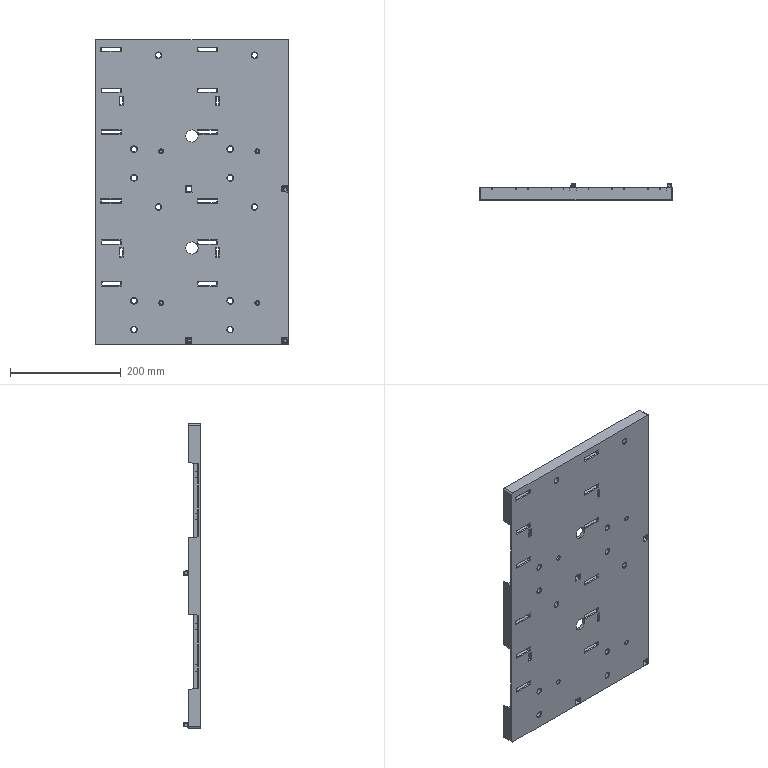Part | STEP file | OP070-1 | 1 solid | 2664 faces | box 350 x 30 x 550 mm | volume 865842 mm3 | plane 2099 | cylinder 357 | spline 120 | cone 88 | commonest cylinder face diameters 2 x142 10 x77 1 x64 33 x28 26 x10 4.3 x8